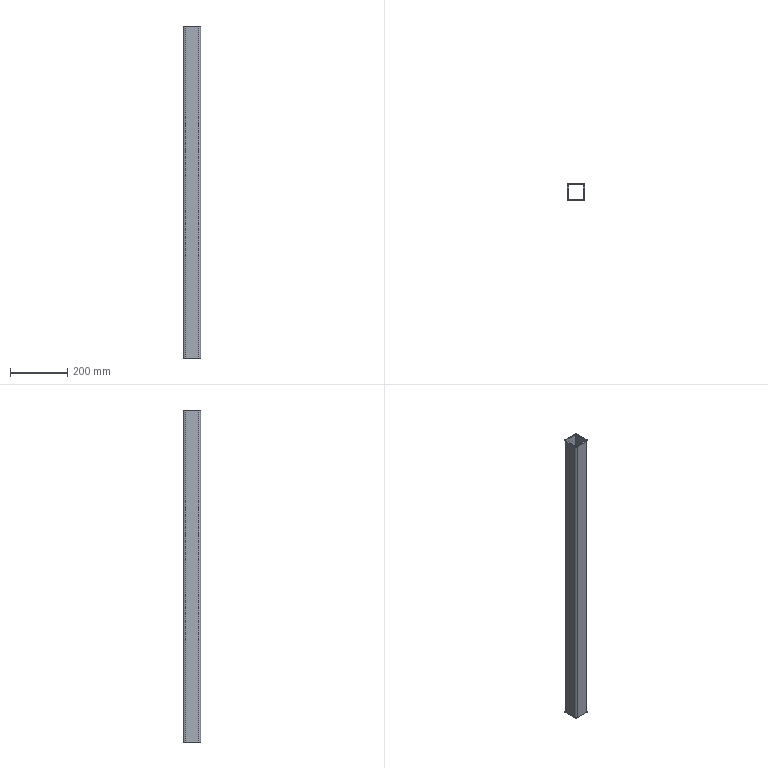Part | STEP file | 750078170 | 1 solid | 18 faces | box 60 x 60 x 1160 mm | volume 1007496 mm3 | plane 10 | cylinder 8 | commonest cylinder face diameters 4 x4 12 x4
STEP:
#1=CARTESIAN_POINT('',(-26.,24.,1160.));
#2=VERTEX_POINT('',#1);
#3=CARTESIAN_POINT('',(-26.,24.,0.));
#4=VERTEX_POINT('',#3);
#5=CARTESIAN_POINT('',(-26.,24.,1160.));
#6=DIRECTION('',(0.,0.,-1.));
#7=VECTOR('',#6,1000.);
#8=LINE('',#5,#7);
#9=EDGE_CURVE('',#2,#4,#8,.T.);
#10=ORIENTED_EDGE('',*,*,#9,.F.);
#11=CARTESIAN_POINT('',(-26.,-24.,1160.));
#12=VERTEX_POINT('',#11);
#13=CARTESIAN_POINT('',(-26.,-24.,1160.));
#14=DIRECTION('',(0.,1.,0.));
#15=VECTOR('',#14,1000.);
#16=LINE('',#13,#15);
#17=EDGE_CURVE('',#12,#2,#16,.T.);
#18=ORIENTED_EDGE('',*,*,#17,.F.);
#19=CARTESIAN_POINT('',(-26.,-24.,0.));
#20=VERTEX_POINT('',#19);
#21=CARTESIAN_POINT('',(-26.,-24.,1160.));
#22=DIRECTION('',(0.,0.,1.));
#23=VECTOR('',#22,1000.);
#24=LINE('',#21,#23);
#25=EDGE_CURVE('',#20,#12,#24,.T.);
#26=ORIENTED_EDGE('',*,*,#25,.F.);
#27=CARTESIAN_POINT('',(-26.,-24.,0.));
#28=DIRECTION('',(0.,-1.,0.));
#29=VECTOR('',#28,1000.);
#30=LINE('',#27,#29);
#31=EDGE_CURVE('',#4,#20,#30,.T.);
#32=ORIENTED_EDGE('',*,*,#31,.F.);
#33=EDGE_LOOP('',(#10,#18,#26,#32));
#34=FACE_OUTER_BOUND('',#33,.T.);
#35=CARTESIAN_POINT('',(-26.,-24.,1160.));
#36=DIRECTION('',(-1.,0.,0.));
#37=DIRECTION('',(0.,-1.,0.));
#38=AXIS2_PLACEMENT_3D('',#35,#36,#37);
#39=PLANE('',#38);
#40=ADVANCED_FACE('',(#34),#39,.F.);
#41=CARTESIAN_POINT('',(26.,24.,0.));
#42=VERTEX_POINT('',#41);
#43=CARTESIAN_POINT('',(24.,26.,0.));
#44=VERTEX_POINT('',#43);
#45=CARTESIAN_POINT('',(24.,24.,0.));
#46=DIRECTION('',(0.,0.,1.));
#47=DIRECTION('',(-1.,0.,0.));
#48=AXIS2_PLACEMENT_3D('',#45,#46,#47);
#49=CIRCLE('',#48,2.);
#50=EDGE_CURVE('',#42,#44,#49,.T.);
#51=ORIENTED_EDGE('',*,*,#50,.T.);
#52=CARTESIAN_POINT('',(-24.,26.,0.));
#53=VERTEX_POINT('',#52);
#54=CARTESIAN_POINT('',(24.,26.,0.));
#55=DIRECTION('',(-1.,0.,0.));
#56=VECTOR('',#55,1000.);
#57=LINE('',#54,#56);
#58=EDGE_CURVE('',#44,#53,#57,.T.);
#59=ORIENTED_EDGE('',*,*,#58,.T.);
#60=CARTESIAN_POINT('',(-24.,24.,0.));
#61=DIRECTION('',(0.,0.,1.));
#62=DIRECTION('',(-1.,0.,0.));
#63=AXIS2_PLACEMENT_3D('',#60,#61,#62);
#64=CIRCLE('',#63,2.);
#65=EDGE_CURVE('',#53,#4,#64,.T.);
#66=ORIENTED_EDGE('',*,*,#65,.T.);
#67=ORIENTED_EDGE('',*,*,#31,.T.);
#68=CARTESIAN_POINT('',(-24.,-26.,0.));
#69=VERTEX_POINT('',#68);
#70=CARTESIAN_POINT('',(-24.,-24.,0.));
#71=DIRECTION('',(0.,0.,1.));
#72=DIRECTION('',(-1.,0.,0.));
#73=AXIS2_PLACEMENT_3D('',#70,#71,#72);
#74=CIRCLE('',#73,2.);
#75=EDGE_CURVE('',#20,#69,#74,.T.);
#76=ORIENTED_EDGE('',*,*,#75,.T.);
#77=CARTESIAN_POINT('',(24.,-26.,0.));
#78=VERTEX_POINT('',#77);
#79=CARTESIAN_POINT('',(24.,-26.,0.));
#80=DIRECTION('',(1.,0.,0.));
#81=VECTOR('',#80,1000.);
#82=LINE('',#79,#81);
#83=EDGE_CURVE('',#69,#78,#82,.T.);
#84=ORIENTED_EDGE('',*,*,#83,.T.);
#85=CARTESIAN_POINT('',(26.,-24.,0.));
#86=VERTEX_POINT('',#85);
#87=CARTESIAN_POINT('',(24.,-24.,0.));
#88=DIRECTION('',(0.,0.,1.));
#89=DIRECTION('',(-1.,0.,0.));
#90=AXIS2_PLACEMENT_3D('',#87,#88,#89);
#91=CIRCLE('',#90,2.);
#92=EDGE_CURVE('',#78,#86,#91,.T.);
#93=ORIENTED_EDGE('',*,*,#92,.T.);
#94=CARTESIAN_POINT('',(26.,-24.,0.));
#95=DIRECTION('',(0.,1.,0.));
#96=VECTOR('',#95,1000.);
#97=LINE('',#94,#96);
#98=EDGE_CURVE('',#86,#42,#97,.T.);
#99=ORIENTED_EDGE('',*,*,#98,.T.);
#100=EDGE_LOOP('',(#51,#59,#66,#67,#76,#84,#93,#99));
#101=FACE_BOUND('',#100,.T.);
#102=CARTESIAN_POINT('',(-24.,30.,0.));
#103=VERTEX_POINT('',#102);
#104=CARTESIAN_POINT('',(24.,30.,0.));
#105=VERTEX_POINT('',#104);
#106=CARTESIAN_POINT('',(24.,30.,0.));
#107=DIRECTION('',(1.,0.,0.));
#108=VECTOR('',#107,1000.);
#109=LINE('',#106,#108);
#110=EDGE_CURVE('',#103,#105,#109,.T.);
#111=ORIENTED_EDGE('',*,*,#110,.T.);
#112=CARTESIAN_POINT('',(30.,24.,0.));
#113=VERTEX_POINT('',#112);
#114=CARTESIAN_POINT('',(24.,24.,0.));
#115=DIRECTION('',(0.,0.,-1.));
#116=DIRECTION('',(-1.,0.,0.));
#117=AXIS2_PLACEMENT_3D('',#114,#115,#116);
#118=CIRCLE('',#117,6.);
#119=EDGE_CURVE('',#105,#113,#118,.T.);
#120=ORIENTED_EDGE('',*,*,#119,.T.);
#121=CARTESIAN_POINT('',(30.,-24.,0.));
#122=VERTEX_POINT('',#121);
#123=CARTESIAN_POINT('',(30.,-24.,0.));
#124=DIRECTION('',(0.,-1.,0.));
#125=VECTOR('',#124,1000.);
#126=LINE('',#123,#125);
#127=EDGE_CURVE('',#113,#122,#126,.T.);
#128=ORIENTED_EDGE('',*,*,#127,.T.);
#129=CARTESIAN_POINT('',(24.,-30.,0.));
#130=VERTEX_POINT('',#129);
#131=CARTESIAN_POINT('',(24.,-24.,0.));
#132=DIRECTION('',(0.,0.,-1.));
#133=DIRECTION('',(-1.,0.,0.));
#134=AXIS2_PLACEMENT_3D('',#131,#132,#133);
#135=CIRCLE('',#134,6.);
#136=EDGE_CURVE('',#122,#130,#135,.T.);
#137=ORIENTED_EDGE('',*,*,#136,.T.);
#138=CARTESIAN_POINT('',(-24.,-30.,0.));
#139=VERTEX_POINT('',#138);
#140=CARTESIAN_POINT('',(24.,-30.,0.));
#141=DIRECTION('',(-1.,0.,0.));
#142=VECTOR('',#141,1000.);
#143=LINE('',#140,#142);
#144=EDGE_CURVE('',#130,#139,#143,.T.);
#145=ORIENTED_EDGE('',*,*,#144,.T.);
#146=CARTESIAN_POINT('',(-30.,-24.,0.));
#147=VERTEX_POINT('',#146);
#148=CARTESIAN_POINT('',(-24.,-24.,0.));
#149=DIRECTION('',(0.,0.,-1.));
#150=DIRECTION('',(-1.,0.,0.));
#151=AXIS2_PLACEMENT_3D('',#148,#149,#150);
#152=CIRCLE('',#151,6.);
#153=EDGE_CURVE('',#139,#147,#152,.T.);
#154=ORIENTED_EDGE('',*,*,#153,.T.);
#155=CARTESIAN_POINT('',(-30.,24.,0.));
#156=VERTEX_POINT('',#155);
#157=CARTESIAN_POINT('',(-30.,-24.,0.));
#158=DIRECTION('',(0.,1.,0.));
#159=VECTOR('',#158,1000.);
#160=LINE('',#157,#159);
#161=EDGE_CURVE('',#147,#156,#160,.T.);
#162=ORIENTED_EDGE('',*,*,#161,.T.);
#163=CARTESIAN_POINT('',(-24.,24.,0.));
#164=DIRECTION('',(0.,0.,-1.));
#165=DIRECTION('',(-1.,0.,0.));
#166=AXIS2_PLACEMENT_3D('',#163,#164,#165);
#167=CIRCLE('',#166,6.);
#168=EDGE_CURVE('',#156,#103,#167,.T.);
#169=ORIENTED_EDGE('',*,*,#168,.T.);
#170=EDGE_LOOP('',(#111,#120,#128,#137,#145,#154,#162,#169));
#171=FACE_OUTER_BOUND('',#170,.T.);
#172=CARTESIAN_POINT('',(24.,-24.,0.));
#173=DIRECTION('',(0.,0.,-1.));
#174=DIRECTION('',(-1.,0.,0.));
#175=AXIS2_PLACEMENT_3D('',#172,#173,#174);
#176=PLANE('',#175);
#177=ADVANCED_FACE('',(#101,#171),#176,.T.);
#178=CARTESIAN_POINT('',(-24.,26.,1160.));
#179=VERTEX_POINT('',#178);
#180=CARTESIAN_POINT('',(-24.,26.,1160.));
#181=DIRECTION('',(0.,0.,-1.));
#182=VECTOR('',#181,1000.);
#183=LINE('',#180,#182);
#184=EDGE_CURVE('',#179,#53,#183,.T.);
#185=ORIENTED_EDGE('',*,*,#184,.F.);
#186=CARTESIAN_POINT('',(-24.,24.,1160.));
#187=DIRECTION('',(0.,0.,-1.));
#188=DIRECTION('',(-1.,0.,0.));
#189=AXIS2_PLACEMENT_3D('',#186,#187,#188);
#190=CIRCLE('',#189,2.);
#191=EDGE_CURVE('',#2,#179,#190,.T.);
#192=ORIENTED_EDGE('',*,*,#191,.F.);
#193=ORIENTED_EDGE('',*,*,#9,.T.);
#194=ORIENTED_EDGE('',*,*,#65,.F.);
#195=EDGE_LOOP('',(#185,#192,#193,#194));
#196=FACE_OUTER_BOUND('',#195,.T.);
#197=CARTESIAN_POINT('',(-24.,24.,1160.));
#198=DIRECTION('',(0.,0.,-1.));
#199=DIRECTION('',(-1.,0.,0.));
#200=AXIS2_PLACEMENT_3D('',#197,#198,#199);
#201=CYLINDRICAL_SURFACE('',#200,2.);
#202=ADVANCED_FACE('',(#196),#201,.F.);
#203=CARTESIAN_POINT('',(24.,26.,1160.));
#204=VERTEX_POINT('',#203);
#205=CARTESIAN_POINT('',(24.,26.,1160.));
#206=DIRECTION('',(-1.,0.,0.));
#207=VECTOR('',#206,1000.);
#208=LINE('',#205,#207);
#209=EDGE_CURVE('',#204,#179,#208,.T.);
#210=ORIENTED_EDGE('',*,*,#209,.F.);
#211=CARTESIAN_POINT('',(26.,24.,1160.));
#212=VERTEX_POINT('',#211);
#213=CARTESIAN_POINT('',(24.,24.,1160.));
#214=DIRECTION('',(0.,0.,1.));
#215=DIRECTION('',(-1.,0.,0.));
#216=AXIS2_PLACEMENT_3D('',#213,#214,#215);
#217=CIRCLE('',#216,2.);
#218=EDGE_CURVE('',#212,#204,#217,.T.);
#219=ORIENTED_EDGE('',*,*,#218,.F.);
#220=CARTESIAN_POINT('',(26.,-24.,1160.));
#221=VERTEX_POINT('',#220);
#222=CARTESIAN_POINT('',(26.,-24.,1160.));
#223=DIRECTION('',(0.,1.,0.));
#224=VECTOR('',#223,1000.);
#225=LINE('',#222,#224);
#226=EDGE_CURVE('',#221,#212,#225,.T.);
#227=ORIENTED_EDGE('',*,*,#226,.F.);
#228=CARTESIAN_POINT('',(24.,-26.,1160.));
#229=VERTEX_POINT('',#228);
#230=CARTESIAN_POINT('',(24.,-24.,1160.));
#231=DIRECTION('',(0.,0.,1.));
#232=DIRECTION('',(-1.,0.,0.));
#233=AXIS2_PLACEMENT_3D('',#230,#231,#232);
#234=CIRCLE('',#233,2.);
#235=EDGE_CURVE('',#229,#221,#234,.T.);
#236=ORIENTED_EDGE('',*,*,#235,.F.);
#237=CARTESIAN_POINT('',(-24.,-26.,1160.));
#238=VERTEX_POINT('',#237);
#239=CARTESIAN_POINT('',(24.,-26.,1160.));
#240=DIRECTION('',(1.,0.,0.));
#241=VECTOR('',#240,1000.);
#242=LINE('',#239,#241);
#243=EDGE_CURVE('',#238,#229,#242,.T.);
#244=ORIENTED_EDGE('',*,*,#243,.F.);
#245=CARTESIAN_POINT('',(-24.,-24.,1160.));
#246=DIRECTION('',(0.,0.,1.));
#247=DIRECTION('',(-1.,0.,0.));
#248=AXIS2_PLACEMENT_3D('',#245,#246,#247);
#249=CIRCLE('',#248,2.);
#250=EDGE_CURVE('',#12,#238,#249,.T.);
#251=ORIENTED_EDGE('',*,*,#250,.F.);
#252=ORIENTED_EDGE('',*,*,#17,.T.);
#253=ORIENTED_EDGE('',*,*,#191,.T.);
#254=EDGE_LOOP('',(#210,#219,#227,#236,#244,#251,#252,#253));
#255=FACE_BOUND('',#254,.T.);
#256=CARTESIAN_POINT('',(24.,30.,1160.));
#257=VERTEX_POINT('',#256);
#258=CARTESIAN_POINT('',(30.,24.,1160.));
#259=VERTEX_POINT('',#258);
#260=CARTESIAN_POINT('',(24.,24.,1160.));
#261=DIRECTION('',(0.,0.,-1.));
#262=DIRECTION('',(-1.,0.,0.));
#263=AXIS2_PLACEMENT_3D('',#260,#261,#262);
#264=CIRCLE('',#263,6.);
#265=EDGE_CURVE('',#257,#259,#264,.T.);
#266=ORIENTED_EDGE('',*,*,#265,.F.);
#267=CARTESIAN_POINT('',(-24.,30.,1160.));
#268=VERTEX_POINT('',#267);
#269=CARTESIAN_POINT('',(24.,30.,1160.));
#270=DIRECTION('',(1.,0.,0.));
#271=VECTOR('',#270,1000.);
#272=LINE('',#269,#271);
#273=EDGE_CURVE('',#268,#257,#272,.T.);
#274=ORIENTED_EDGE('',*,*,#273,.F.);
#275=CARTESIAN_POINT('',(-30.,24.,1160.));
#276=VERTEX_POINT('',#275);
#277=CARTESIAN_POINT('',(-24.,24.,1160.));
#278=DIRECTION('',(0.,0.,-1.));
#279=DIRECTION('',(-1.,0.,0.));
#280=AXIS2_PLACEMENT_3D('',#277,#278,#279);
#281=CIRCLE('',#280,6.);
#282=EDGE_CURVE('',#276,#268,#281,.T.);
#283=ORIENTED_EDGE('',*,*,#282,.F.);
#284=CARTESIAN_POINT('',(-30.,-24.,1160.));
#285=VERTEX_POINT('',#284);
#286=CARTESIAN_POINT('',(-30.,-24.,1160.));
#287=DIRECTION('',(0.,1.,0.));
#288=VECTOR('',#287,1000.);
#289=LINE('',#286,#288);
#290=EDGE_CURVE('',#285,#276,#289,.T.);
#291=ORIENTED_EDGE('',*,*,#290,.F.);
#292=CARTESIAN_POINT('',(-24.,-30.,1160.));
#293=VERTEX_POINT('',#292);
#294=CARTESIAN_POINT('',(-24.,-24.,1160.));
#295=DIRECTION('',(0.,0.,-1.));
#296=DIRECTION('',(-1.,0.,0.));
#297=AXIS2_PLACEMENT_3D('',#294,#295,#296);
#298=CIRCLE('',#297,6.);
#299=EDGE_CURVE('',#293,#285,#298,.T.);
#300=ORIENTED_EDGE('',*,*,#299,.F.);
#301=CARTESIAN_POINT('',(24.,-30.,1160.));
#302=VERTEX_POINT('',#301);
#303=CARTESIAN_POINT('',(24.,-30.,1160.));
#304=DIRECTION('',(-1.,0.,0.));
#305=VECTOR('',#304,1000.);
#306=LINE('',#303,#305);
#307=EDGE_CURVE('',#302,#293,#306,.T.);
#308=ORIENTED_EDGE('',*,*,#307,.F.);
#309=CARTESIAN_POINT('',(30.,-24.,1160.));
#310=VERTEX_POINT('',#309);
#311=CARTESIAN_POINT('',(24.,-24.,1160.));
#312=DIRECTION('',(0.,0.,-1.));
#313=DIRECTION('',(-1.,0.,0.));
#314=AXIS2_PLACEMENT_3D('',#311,#312,#313);
#315=CIRCLE('',#314,6.);
#316=EDGE_CURVE('',#310,#302,#315,.T.);
#317=ORIENTED_EDGE('',*,*,#316,.F.);
#318=CARTESIAN_POINT('',(30.,-24.,1160.));
#319=DIRECTION('',(0.,-1.,0.));
#320=VECTOR('',#319,1000.);
#321=LINE('',#318,#320);
#322=EDGE_CURVE('',#259,#310,#321,.T.);
#323=ORIENTED_EDGE('',*,*,#322,.F.);
#324=EDGE_LOOP('',(#266,#274,#283,#291,#300,#308,#317,#323));
#325=FACE_OUTER_BOUND('',#324,.T.);
#326=CARTESIAN_POINT('',(24.,-24.,1160.));
#327=DIRECTION('',(0.,0.,-1.));
#328=DIRECTION('',(-1.,0.,0.));
#329=AXIS2_PLACEMENT_3D('',#326,#327,#328);
#330=PLANE('',#329);
#331=ADVANCED_FACE('',(#255,#325),#330,.F.);
#332=ORIENTED_EDGE('',*,*,#25,.T.);
#333=ORIENTED_EDGE('',*,*,#250,.T.);
#334=CARTESIAN_POINT('',(-24.,-26.,1160.));
#335=DIRECTION('',(0.,0.,1.));
#336=VECTOR('',#335,1000.);
#337=LINE('',#334,#336);
#338=EDGE_CURVE('',#69,#238,#337,.T.);
#339=ORIENTED_EDGE('',*,*,#338,.F.);
#340=ORIENTED_EDGE('',*,*,#75,.F.);
#341=EDGE_LOOP('',(#332,#333,#339,#340));
#342=FACE_OUTER_BOUND('',#341,.T.);
#343=CARTESIAN_POINT('',(-24.,-24.,1160.));
#344=DIRECTION('',(0.,0.,-1.));
#345=DIRECTION('',(-1.,0.,0.));
#346=AXIS2_PLACEMENT_3D('',#343,#344,#345);
#347=CYLINDRICAL_SURFACE('',#346,2.);
#348=ADVANCED_FACE('',(#342),#347,.F.);
#349=CARTESIAN_POINT('',(24.,26.,1160.));
#350=DIRECTION('',(0.,0.,-1.));
#351=VECTOR('',#350,1000.);
#352=LINE('',#349,#351);
#353=EDGE_CURVE('',#204,#44,#352,.T.);
#354=ORIENTED_EDGE('',*,*,#353,.F.);
#355=ORIENTED_EDGE('',*,*,#209,.T.);
#356=ORIENTED_EDGE('',*,*,#184,.T.);
#357=ORIENTED_EDGE('',*,*,#58,.F.);
#358=EDGE_LOOP('',(#354,#355,#356,#357));
#359=FACE_OUTER_BOUND('',#358,.T.);
#360=CARTESIAN_POINT('',(-24.,26.,1160.));
#361=DIRECTION('',(0.,1.,0.));
#362=DIRECTION('',(0.,0.,1.));
#363=AXIS2_PLACEMENT_3D('',#360,#361,#362);
#364=PLANE('',#363);
#365=ADVANCED_FACE('',(#359),#364,.F.);
#366=CARTESIAN_POINT('',(26.,24.,1160.));
#367=DIRECTION('',(0.,0.,-1.));
#368=VECTOR('',#367,1000.);
#369=LINE('',#366,#368);
#370=EDGE_CURVE('',#212,#42,#369,.T.);
#371=ORIENTED_EDGE('',*,*,#370,.F.);
#372=ORIENTED_EDGE('',*,*,#218,.T.);
#373=ORIENTED_EDGE('',*,*,#353,.T.);
#374=ORIENTED_EDGE('',*,*,#50,.F.);
#375=EDGE_LOOP('',(#371,#372,#373,#374));
#376=FACE_OUTER_BOUND('',#375,.T.);
#377=CARTESIAN_POINT('',(24.,24.,1160.));
#378=DIRECTION('',(0.,0.,-1.));
#379=DIRECTION('',(-1.,0.,0.));
#380=AXIS2_PLACEMENT_3D('',#377,#378,#379);
#381=CYLINDRICAL_SURFACE('',#380,2.);
#382=ADVANCED_FACE('',(#376),#381,.F.);
#383=CARTESIAN_POINT('',(26.,-24.,1160.));
#384=DIRECTION('',(0.,0.,-1.));
#385=VECTOR('',#384,1000.);
#386=LINE('',#383,#385);
#387=EDGE_CURVE('',#221,#86,#386,.T.);
#388=ORIENTED_EDGE('',*,*,#387,.F.);
#389=ORIENTED_EDGE('',*,*,#226,.T.);
#390=ORIENTED_EDGE('',*,*,#370,.T.);
#391=ORIENTED_EDGE('',*,*,#98,.F.);
#392=EDGE_LOOP('',(#388,#389,#390,#391));
#393=FACE_OUTER_BOUND('',#392,.T.);
#394=CARTESIAN_POINT('',(26.,24.,1160.));
#395=DIRECTION('',(1.,0.,0.));
#396=DIRECTION('',(0.,0.,-1.));
#397=AXIS2_PLACEMENT_3D('',#394,#395,#396);
#398=PLANE('',#397);
#399=ADVANCED_FACE('',(#393),#398,.F.);
#400=CARTESIAN_POINT('',(24.,-26.,1160.));
#401=DIRECTION('',(0.,0.,-1.));
#402=VECTOR('',#401,1000.);
#403=LINE('',#400,#402);
#404=EDGE_CURVE('',#229,#78,#403,.T.);
#405=ORIENTED_EDGE('',*,*,#404,.F.);
#406=ORIENTED_EDGE('',*,*,#235,.T.);
#407=ORIENTED_EDGE('',*,*,#387,.T.);
#408=ORIENTED_EDGE('',*,*,#92,.F.);
#409=EDGE_LOOP('',(#405,#406,#407,#408));
#410=FACE_OUTER_BOUND('',#409,.T.);
#411=CARTESIAN_POINT('',(24.,-24.,1160.));
#412=DIRECTION('',(0.,0.,-1.));
#413=DIRECTION('',(-1.,0.,0.));
#414=AXIS2_PLACEMENT_3D('',#411,#412,#413);
#415=CYLINDRICAL_SURFACE('',#414,2.);
#416=ADVANCED_FACE('',(#410),#415,.F.);
#417=ORIENTED_EDGE('',*,*,#338,.T.);
#418=ORIENTED_EDGE('',*,*,#243,.T.);
#419=ORIENTED_EDGE('',*,*,#404,.T.);
#420=ORIENTED_EDGE('',*,*,#83,.F.);
#421=EDGE_LOOP('',(#417,#418,#419,#420));
#422=FACE_OUTER_BOUND('',#421,.T.);
#423=CARTESIAN_POINT('',(24.,-26.,1160.));
#424=DIRECTION('',(0.,-1.,0.));
#425=DIRECTION('',(0.,0.,-1.));
#426=AXIS2_PLACEMENT_3D('',#423,#424,#425);
#427=PLANE('',#426);
#428=ADVANCED_FACE('',(#422),#427,.F.);
#429=ORIENTED_EDGE('',*,*,#265,.T.);
#430=CARTESIAN_POINT('',(30.,24.,1160.));
#431=DIRECTION('',(0.,0.,-1.));
#432=VECTOR('',#431,1000.);
#433=LINE('',#430,#432);
#434=EDGE_CURVE('',#259,#113,#433,.T.);
#435=ORIENTED_EDGE('',*,*,#434,.T.);
#436=ORIENTED_EDGE('',*,*,#119,.F.);
#437=CARTESIAN_POINT('',(24.,30.,1160.));
#438=DIRECTION('',(0.,0.,1.));
#439=VECTOR('',#438,1000.);
#440=LINE('',#437,#439);
#441=EDGE_CURVE('',#105,#257,#440,.T.);
#442=ORIENTED_EDGE('',*,*,#441,.T.);
#443=EDGE_LOOP('',(#429,#435,#436,#442));
#444=FACE_OUTER_BOUND('',#443,.T.);
#445=CARTESIAN_POINT('',(24.,24.,1160.));
#446=DIRECTION('',(0.,0.,-1.));
#447=DIRECTION('',(-1.,0.,0.));
#448=AXIS2_PLACEMENT_3D('',#445,#446,#447);
#449=CYLINDRICAL_SURFACE('',#448,6.);
#450=ADVANCED_FACE('',(#444),#449,.T.);
#451=ORIENTED_EDGE('',*,*,#273,.T.);
#452=ORIENTED_EDGE('',*,*,#441,.F.);
#453=ORIENTED_EDGE('',*,*,#110,.F.);
#454=CARTESIAN_POINT('',(-24.,30.,1160.));
#455=DIRECTION('',(0.,0.,1.));
#456=VECTOR('',#455,1000.);
#457=LINE('',#454,#456);
#458=EDGE_CURVE('',#103,#268,#457,.T.);
#459=ORIENTED_EDGE('',*,*,#458,.T.);
#460=EDGE_LOOP('',(#451,#452,#453,#459));
#461=FACE_OUTER_BOUND('',#460,.T.);
#462=CARTESIAN_POINT('',(-24.,30.,1160.));
#463=DIRECTION('',(0.,1.,0.));
#464=DIRECTION('',(-1.,0.,0.));
#465=AXIS2_PLACEMENT_3D('',#462,#463,#464);
#466=PLANE('',#465);
#467=ADVANCED_FACE('',(#461),#466,.T.);
#468=ORIENTED_EDGE('',*,*,#282,.T.);
#469=ORIENTED_EDGE('',*,*,#458,.F.);
#470=ORIENTED_EDGE('',*,*,#168,.F.);
#471=CARTESIAN_POINT('',(-30.,24.,1160.));
#472=DIRECTION('',(0.,0.,1.));
#473=VECTOR('',#472,1000.);
#474=LINE('',#471,#473);
#475=EDGE_CURVE('',#156,#276,#474,.T.);
#476=ORIENTED_EDGE('',*,*,#475,.T.);
#477=EDGE_LOOP('',(#468,#469,#470,#476));
#478=FACE_OUTER_BOUND('',#477,.T.);
#479=CARTESIAN_POINT('',(-24.,24.,1160.));
#480=DIRECTION('',(0.,0.,-1.));
#481=DIRECTION('',(-1.,0.,0.));
#482=AXIS2_PLACEMENT_3D('',#479,#480,#481);
#483=CYLINDRICAL_SURFACE('',#482,6.);
#484=ADVANCED_FACE('',(#478),#483,.T.);
#485=ORIENTED_EDGE('',*,*,#290,.T.);
#486=ORIENTED_EDGE('',*,*,#475,.F.);
#487=ORIENTED_EDGE('',*,*,#161,.F.);
#488=CARTESIAN_POINT('',(-30.,-24.,1160.));
#489=DIRECTION('',(0.,0.,1.));
#490=VECTOR('',#489,1000.);
#491=LINE('',#488,#490);
#492=EDGE_CURVE('',#147,#285,#491,.T.);
#493=ORIENTED_EDGE('',*,*,#492,.T.);
#494=EDGE_LOOP('',(#485,#486,#487,#493));
#495=FACE_OUTER_BOUND('',#494,.T.);
#496=CARTESIAN_POINT('',(-30.,-24.,1160.));
#497=DIRECTION('',(-1.,0.,0.));
#498=DIRECTION('',(0.,-1.,0.));
#499=AXIS2_PLACEMENT_3D('',#496,#497,#498);
#500=PLANE('',#499);
#501=ADVANCED_FACE('',(#495),#500,.T.);
#502=ORIENTED_EDGE('',*,*,#299,.T.);
#503=ORIENTED_EDGE('',*,*,#492,.F.);
#504=ORIENTED_EDGE('',*,*,#153,.F.);
#505=CARTESIAN_POINT('',(-24.,-30.,1160.));
#506=DIRECTION('',(0.,0.,1.));
#507=VECTOR('',#506,1000.);
#508=LINE('',#505,#507);
#509=EDGE_CURVE('',#139,#293,#508,.T.);
#510=ORIENTED_EDGE('',*,*,#509,.T.);
#511=EDGE_LOOP('',(#502,#503,#504,#510));
#512=FACE_OUTER_BOUND('',#511,.T.);
#513=CARTESIAN_POINT('',(-24.,-24.,1160.));
#514=DIRECTION('',(0.,0.,-1.));
#515=DIRECTION('',(-1.,0.,0.));
#516=AXIS2_PLACEMENT_3D('',#513,#514,#515);
#517=CYLINDRICAL_SURFACE('',#516,6.);
#518=ADVANCED_FACE('',(#512),#517,.T.);
#519=ORIENTED_EDGE('',*,*,#307,.T.);
#520=ORIENTED_EDGE('',*,*,#509,.F.);
#521=ORIENTED_EDGE('',*,*,#144,.F.);
#522=CARTESIAN_POINT('',(24.,-30.,1160.));
#523=DIRECTION('',(0.,0.,1.));
#524=VECTOR('',#523,1000.);
#525=LINE('',#522,#524);
#526=EDGE_CURVE('',#130,#302,#525,.T.);
#527=ORIENTED_EDGE('',*,*,#526,.T.);
#528=EDGE_LOOP('',(#519,#520,#521,#527));
#529=FACE_OUTER_BOUND('',#528,.T.);
#530=CARTESIAN_POINT('',(24.,-30.,1160.));
#531=DIRECTION('',(0.,-1.,0.));
#532=DIRECTION('',(1.,0.,0.));
#533=AXIS2_PLACEMENT_3D('',#530,#531,#532);
#534=PLANE('',#533);
#535=ADVANCED_FACE('',(#529),#534,.T.);
#536=ORIENTED_EDGE('',*,*,#316,.T.);
#537=ORIENTED_EDGE('',*,*,#526,.F.);
#538=ORIENTED_EDGE('',*,*,#136,.F.);
#539=CARTESIAN_POINT('',(30.,-24.,1160.));
#540=DIRECTION('',(0.,0.,1.));
#541=VECTOR('',#540,1000.);
#542=LINE('',#539,#541);
#543=EDGE_CURVE('',#122,#310,#542,.T.);
#544=ORIENTED_EDGE('',*,*,#543,.T.);
#545=EDGE_LOOP('',(#536,#537,#538,#544));
#546=FACE_OUTER_BOUND('',#545,.T.);
#547=CARTESIAN_POINT('',(24.,-24.,1160.));
#548=DIRECTION('',(0.,0.,-1.));
#549=DIRECTION('',(-1.,0.,0.));
#550=AXIS2_PLACEMENT_3D('',#547,#548,#549);
#551=CYLINDRICAL_SURFACE('',#550,6.);
#552=ADVANCED_FACE('',(#546),#551,.T.);
#553=ORIENTED_EDGE('',*,*,#322,.T.);
#554=ORIENTED_EDGE('',*,*,#543,.F.);
#555=ORIENTED_EDGE('',*,*,#127,.F.);
#556=ORIENTED_EDGE('',*,*,#434,.F.);
#557=EDGE_LOOP('',(#553,#554,#555,#556));
#558=FACE_OUTER_BOUND('',#557,.T.);
#559=CARTESIAN_POINT('',(30.,24.,1160.));
#560=DIRECTION('',(1.,0.,0.));
#561=DIRECTION('',(0.,0.,-1.));
#562=AXIS2_PLACEMENT_3D('',#559,#560,#561);
#563=PLANE('',#562);
#564=ADVANCED_FACE('',(#558),#563,.T.);
#565=CLOSED_SHELL('',(#40,#177,#202,#331,#348,#365,#382,#399,#416,#428,#450,#467,#484,#501,#518,#535,#552,#564));
#566=MANIFOLD_SOLID_BREP('',#565);
#567=CARTESIAN_POINT('',(0.,0.,0.));
#568=DIRECTION('',(0.,0.,1.));
#569=DIRECTION('',(1.,0.,0.));
#570=AXIS2_PLACEMENT_3D('',#567,#568,#569);
#571=(LENGTH_UNIT()NAMED_UNIT(*)SI_UNIT(.MILLI.,.METRE.));
#572=UNCERTAINTY_MEASURE_WITH_UNIT(LENGTH_MEASURE(0.00001),#571,'','');
#573=(NAMED_UNIT(*)PLANE_ANGLE_UNIT()SI_UNIT($,.RADIAN.));
#574=(NAMED_UNIT(*)SI_UNIT($,.STERADIAN.)SOLID_ANGLE_UNIT());
#575=(GEOMETRIC_REPRESENTATION_CONTEXT(3)GLOBAL_UNCERTAINTY_ASSIGNED_CONTEXT((#572))GLOBAL_UNIT_ASSIGNED_CONTEXT((#571,#573,#574))REPRESENTATION_CONTEXT('',''));
#576=ADVANCED_BREP_SHAPE_REPRESENTATION('',(#566,#570),#575);